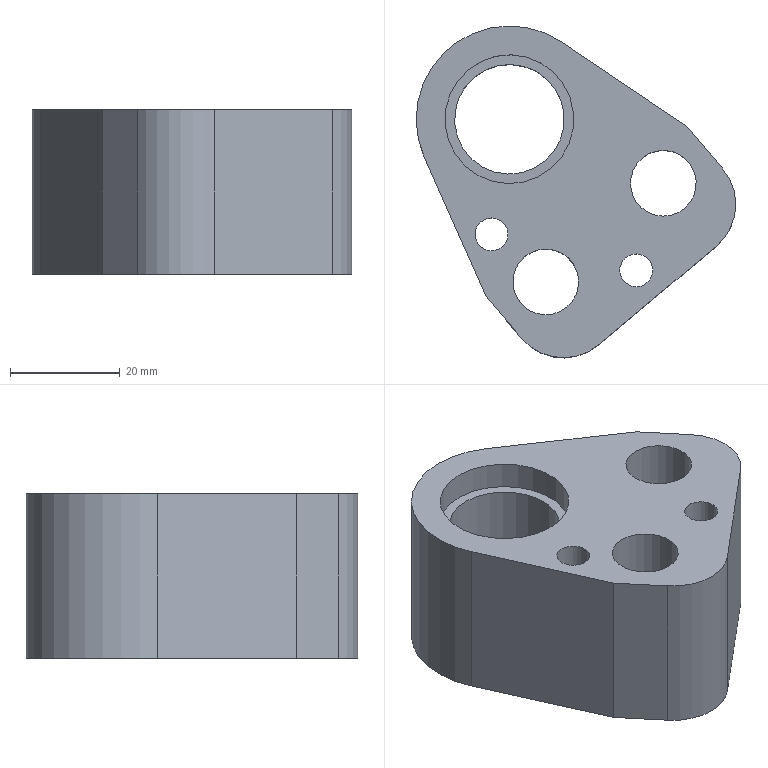Part | NX | features solid 2 | 1 solid | 25 faces | box 58.294 x 60.512 x 30 mm | volume 46591 mm3 | cylinder 13 | plane 12 | commonest cylinder face diameters 20 x3 6 x2 8 x2 12 x2 17 x2 23.5 x1
STEP:
#1=CARTESIAN_POINT('',(142.417,-221.513,161.));
#2=VERTEX_POINT('',#1);
#3=CARTESIAN_POINT('',(144.989,-224.578,161.));
#4=DIRECTION('',(0.,0.,-1.));
#5=DIRECTION('',(-0.6428,0.766,0.));
#6=AXIS2_PLACEMENT_3D('',#3,#4,#5);
#7=CIRCLE('',#6,4.);
#8=EDGE_CURVE('',#2,#2,#7,.F.);
#9=ORIENTED_EDGE('',*,*,#8,.T.);
#10=EDGE_LOOP('',(#9));
#11=FACE_BOUND('',#10,.T.);
#12=CARTESIAN_POINT('',(133.943,-233.194,161.));
#13=VERTEX_POINT('',#12);
#14=CARTESIAN_POINT('',(128.479,-226.682,161.));
#15=DIRECTION('',(0.,0.,1.));
#16=DIRECTION('',(0.6428,-0.766,0.));
#17=AXIS2_PLACEMENT_3D('',#14,#15,#16);
#18=CIRCLE('',#17,8.5);
#19=EDGE_CURVE('',#13,#13,#18,.T.);
#20=ORIENTED_EDGE('',*,*,#19,.T.);
#21=EDGE_LOOP('',(#20));
#22=FACE_BOUND('',#21,.T.);
#23=CARTESIAN_POINT('',(155.392,-215.196,161.));
#24=VERTEX_POINT('',#23);
#25=CARTESIAN_POINT('',(149.928,-208.684,161.));
#26=DIRECTION('',(0.,0.,1.));
#27=DIRECTION('',(0.6428,-0.766,0.));
#28=AXIS2_PLACEMENT_3D('',#25,#26,#27);
#29=CIRCLE('',#28,8.5);
#30=EDGE_CURVE('',#24,#24,#29,.T.);
#31=ORIENTED_EDGE('',*,*,#30,.T.);
#32=EDGE_LOOP('',(#31));
#33=FACE_BOUND('',#32,.T.);
#34=CARTESIAN_POINT('',(115.42,-189.34,161.));
#35=VERTEX_POINT('',#34);
#36=CARTESIAN_POINT('',(121.848,-197.,161.));
#37=DIRECTION('',(0.,0.,-1.));
#38=DIRECTION('',(-0.6428,0.766,0.));
#39=AXIS2_PLACEMENT_3D('',#36,#37,#38);
#40=CIRCLE('',#39,10.);
#41=EDGE_CURVE('',#35,#35,#40,.T.);
#42=ORIENTED_EDGE('',*,*,#41,.F.);
#43=EDGE_LOOP('',(#42));
#44=FACE_BOUND('',#43,.T.);
#45=CARTESIAN_POINT('',(131.351,-182.904,161.));
#46=VERTEX_POINT('',#45);
#47=CARTESIAN_POINT('',(154.375,-198.426,161.));
#48=VERTEX_POINT('',#47);
#49=CARTESIAN_POINT('',(131.351,-182.904,161.));
#50=DIRECTION('',(0.8292,-0.559,0.));
#51=VECTOR('',#50,1000.);
#52=LINE('',#49,#51);
#53=EDGE_CURVE('',#46,#48,#52,.T.);
#54=ORIENTED_EDGE('',*,*,#53,.T.);
#55=CARTESIAN_POINT('',(160.803,-206.087,161.));
#56=VERTEX_POINT('',#55);
#57=CARTESIAN_POINT('',(154.375,-198.426,161.));
#58=DIRECTION('',(0.6428,-0.766,0.));
#59=VECTOR('',#58,1000.);
#60=LINE('',#57,#59);
#61=EDGE_CURVE('',#48,#56,#60,.T.);
#62=ORIENTED_EDGE('',*,*,#61,.T.);
#63=CARTESIAN_POINT('',(159.57,-220.175,161.));
#64=VERTEX_POINT('',#63);
#65=CARTESIAN_POINT('',(153.142,-212.514,161.));
#66=DIRECTION('',(0.,0.,1.));
#67=DIRECTION('',(0.6428,-0.766,0.));
#68=AXIS2_PLACEMENT_3D('',#65,#66,#67);
#69=CIRCLE('',#68,10.);
#70=EDGE_CURVE('',#64,#56,#69,.T.);
#71=ORIENTED_EDGE('',*,*,#70,.F.);
#72=CARTESIAN_POINT('',(138.121,-238.173,161.));
#73=VERTEX_POINT('',#72);
#74=CARTESIAN_POINT('',(159.57,-220.175,161.));
#75=DIRECTION('',(-0.766,-0.6428,0.));
#76=VECTOR('',#75,1000.);
#77=LINE('',#74,#76);
#78=EDGE_CURVE('',#64,#73,#77,.T.);
#79=ORIENTED_EDGE('',*,*,#78,.T.);
#80=CARTESIAN_POINT('',(124.032,-236.94,161.));
#81=VERTEX_POINT('',#80);
#82=CARTESIAN_POINT('',(131.693,-230.512,161.));
#83=DIRECTION('',(0.,0.,1.));
#84=DIRECTION('',(0.6428,-0.766,0.));
#85=AXIS2_PLACEMENT_3D('',#82,#83,#84);
#86=CIRCLE('',#85,10.);
#87=EDGE_CURVE('',#81,#73,#86,.T.);
#88=ORIENTED_EDGE('',*,*,#87,.F.);
#89=CARTESIAN_POINT('',(117.605,-229.28,161.));
#90=VERTEX_POINT('',#89);
#91=CARTESIAN_POINT('',(117.605,-229.28,161.));
#92=DIRECTION('',(0.6428,-0.766,0.));
#93=VECTOR('',#92,1000.);
#94=LINE('',#91,#93);
#95=EDGE_CURVE('',#90,#81,#94,.T.);
#96=ORIENTED_EDGE('',*,*,#95,.F.);
#97=CARTESIAN_POINT('',(106.316,-203.911,161.));
#98=VERTEX_POINT('',#97);
#99=CARTESIAN_POINT('',(106.316,-203.911,161.));
#100=DIRECTION('',(0.4065,-0.9136,0.));
#101=VECTOR('',#100,1000.);
#102=LINE('',#99,#101);
#103=EDGE_CURVE('',#98,#90,#102,.T.);
#104=ORIENTED_EDGE('',*,*,#103,.F.);
#105=CARTESIAN_POINT('',(121.848,-197.,161.));
#106=DIRECTION('',(0.,0.,1.));
#107=DIRECTION('',(0.6428,-0.766,0.));
#108=AXIS2_PLACEMENT_3D('',#105,#106,#107);
#109=CIRCLE('',#108,17.);
#110=EDGE_CURVE('',#46,#98,#109,.T.);
#111=ORIENTED_EDGE('',*,*,#110,.F.);
#112=EDGE_LOOP('',(#54,#62,#71,#79,#88,#96,#104,#111));
#113=FACE_BOUND('',#112,.T.);
#114=CARTESIAN_POINT('',(116.019,-214.945,161.));
#115=VERTEX_POINT('',#114);
#116=CARTESIAN_POINT('',(118.591,-218.009,161.));
#117=DIRECTION('',(0.,0.,-1.));
#118=DIRECTION('',(-0.6428,0.766,0.));
#119=AXIS2_PLACEMENT_3D('',#116,#117,#118);
#120=CIRCLE('',#119,4.);
#121=EDGE_CURVE('',#115,#115,#120,.F.);
#122=ORIENTED_EDGE('',*,*,#121,.T.);
#123=EDGE_LOOP('',(#122));
#124=FACE_BOUND('',#123,.T.);
#125=CARTESIAN_POINT('',(153.142,-212.514,161.));
#126=DIRECTION('',(0.,0.,-1.));
#127=DIRECTION('',(0.6428,-0.766,0.));
#128=AXIS2_PLACEMENT_3D('',#125,#126,#127);
#129=PLANE('',#128);
#130=ADVANCED_FACE('',(#11,#22,#33,#44,#113,#124),#129,.T.);
#131=CARTESIAN_POINT('',(146.917,-226.876,191.));
#132=VERTEX_POINT('',#131);
#133=CARTESIAN_POINT('',(144.989,-224.578,191.));
#134=DIRECTION('',(0.,0.,1.));
#135=DIRECTION('',(0.6428,-0.766,0.));
#136=AXIS2_PLACEMENT_3D('',#133,#134,#135);
#137=CIRCLE('',#136,3.);
#138=EDGE_CURVE('',#132,#132,#137,.T.);
#139=ORIENTED_EDGE('',*,*,#138,.T.);
#140=EDGE_LOOP('',(#139));
#141=FACE_BOUND('',#140,.T.);
#142=CARTESIAN_POINT('',(146.917,-226.876,181.));
#143=VERTEX_POINT('',#142);
#144=CARTESIAN_POINT('',(144.989,-224.578,181.));
#145=DIRECTION('',(0.,0.,1.));
#146=DIRECTION('',(0.6428,-0.766,0.));
#147=AXIS2_PLACEMENT_3D('',#144,#145,#146);
#148=CIRCLE('',#147,3.);
#149=EDGE_CURVE('',#143,#143,#148,.T.);
#150=ORIENTED_EDGE('',*,*,#149,.F.);
#151=EDGE_LOOP('',(#150));
#152=FACE_BOUND('',#151,.T.);
#153=CARTESIAN_POINT('',(144.989,-224.578,161.));
#154=DIRECTION('',(0.,0.,1.));
#155=DIRECTION('',(-0.6428,0.766,0.));
#156=AXIS2_PLACEMENT_3D('',#153,#154,#155);
#157=CYLINDRICAL_SURFACE('',#156,3.);
#158=ADVANCED_FACE('',(#141,#152),#157,.F.);
#159=CARTESIAN_POINT('',(132.336,-231.278,191.));
#160=VERTEX_POINT('',#159);
#161=CARTESIAN_POINT('',(128.479,-226.682,191.));
#162=DIRECTION('',(0.,0.,1.));
#163=DIRECTION('',(0.6428,-0.766,0.));
#164=AXIS2_PLACEMENT_3D('',#161,#162,#163);
#165=CIRCLE('',#164,6.);
#166=EDGE_CURVE('',#160,#160,#165,.T.);
#167=ORIENTED_EDGE('',*,*,#166,.T.);
#168=EDGE_LOOP('',(#167));
#169=FACE_BOUND('',#168,.T.);
#170=CARTESIAN_POINT('',(132.336,-231.278,173.));
#171=VERTEX_POINT('',#170);
#172=CARTESIAN_POINT('',(128.479,-226.682,173.));
#173=DIRECTION('',(0.,0.,1.));
#174=DIRECTION('',(0.6428,-0.766,0.));
#175=AXIS2_PLACEMENT_3D('',#172,#173,#174);
#176=CIRCLE('',#175,6.);
#177=EDGE_CURVE('',#171,#171,#176,.T.);
#178=ORIENTED_EDGE('',*,*,#177,.F.);
#179=EDGE_LOOP('',(#178));
#180=FACE_BOUND('',#179,.T.);
#181=CARTESIAN_POINT('',(128.479,-226.682,161.));
#182=DIRECTION('',(0.,0.,1.));
#183=DIRECTION('',(-0.6428,0.766,0.));
#184=AXIS2_PLACEMENT_3D('',#181,#182,#183);
#185=CYLINDRICAL_SURFACE('',#184,6.);
#186=ADVANCED_FACE('',(#169,#180),#185,.F.);
#187=CARTESIAN_POINT('',(153.785,-213.28,191.));
#188=VERTEX_POINT('',#187);
#189=CARTESIAN_POINT('',(149.928,-208.684,191.));
#190=DIRECTION('',(0.,0.,1.));
#191=DIRECTION('',(0.6428,-0.766,0.));
#192=AXIS2_PLACEMENT_3D('',#189,#190,#191);
#193=CIRCLE('',#192,6.);
#194=EDGE_CURVE('',#188,#188,#193,.T.);
#195=ORIENTED_EDGE('',*,*,#194,.T.);
#196=EDGE_LOOP('',(#195));
#197=FACE_BOUND('',#196,.T.);
#198=CARTESIAN_POINT('',(153.785,-213.28,173.));
#199=VERTEX_POINT('',#198);
#200=CARTESIAN_POINT('',(149.928,-208.684,173.));
#201=DIRECTION('',(0.,0.,1.));
#202=DIRECTION('',(0.6428,-0.766,0.));
#203=AXIS2_PLACEMENT_3D('',#200,#201,#202);
#204=CIRCLE('',#203,6.);
#205=EDGE_CURVE('',#199,#199,#204,.T.);
#206=ORIENTED_EDGE('',*,*,#205,.F.);
#207=EDGE_LOOP('',(#206));
#208=FACE_BOUND('',#207,.T.);
#209=CARTESIAN_POINT('',(149.928,-208.684,161.));
#210=DIRECTION('',(0.,0.,1.));
#211=DIRECTION('',(-0.6428,0.766,0.));
#212=AXIS2_PLACEMENT_3D('',#209,#210,#211);
#213=CYLINDRICAL_SURFACE('',#212,6.);
#214=ADVANCED_FACE('',(#197,#208),#213,.F.);
#215=CARTESIAN_POINT('',(120.519,-220.307,191.));
#216=VERTEX_POINT('',#215);
#217=CARTESIAN_POINT('',(118.591,-218.009,191.));
#218=DIRECTION('',(0.,0.,1.));
#219=DIRECTION('',(0.6428,-0.766,0.));
#220=AXIS2_PLACEMENT_3D('',#217,#218,#219);
#221=CIRCLE('',#220,3.);
#222=EDGE_CURVE('',#216,#216,#221,.T.);
#223=ORIENTED_EDGE('',*,*,#222,.F.);
#224=EDGE_LOOP('',(#223));
#225=FACE_BOUND('',#224,.T.);
#226=ORIENTED_EDGE('',*,*,#166,.F.);
#227=EDGE_LOOP('',(#226));
#228=FACE_BOUND('',#227,.T.);
#229=CARTESIAN_POINT('',(131.351,-182.904,191.));
#230=VERTEX_POINT('',#229);
#231=CARTESIAN_POINT('',(154.375,-198.426,191.));
#232=VERTEX_POINT('',#231);
#233=CARTESIAN_POINT('',(131.351,-182.904,191.));
#234=DIRECTION('',(0.8292,-0.559,0.));
#235=VECTOR('',#234,1000.);
#236=LINE('',#233,#235);
#237=EDGE_CURVE('',#230,#232,#236,.T.);
#238=ORIENTED_EDGE('',*,*,#237,.F.);
#239=CARTESIAN_POINT('',(106.316,-203.911,191.));
#240=VERTEX_POINT('',#239);
#241=CARTESIAN_POINT('',(121.848,-197.,191.));
#242=DIRECTION('',(0.,0.,1.));
#243=DIRECTION('',(0.6428,-0.766,0.));
#244=AXIS2_PLACEMENT_3D('',#241,#242,#243);
#245=CIRCLE('',#244,17.);
#246=EDGE_CURVE('',#230,#240,#245,.T.);
#247=ORIENTED_EDGE('',*,*,#246,.T.);
#248=CARTESIAN_POINT('',(117.605,-229.28,191.));
#249=VERTEX_POINT('',#248);
#250=CARTESIAN_POINT('',(106.316,-203.911,191.));
#251=DIRECTION('',(0.4065,-0.9136,0.));
#252=VECTOR('',#251,1000.);
#253=LINE('',#250,#252);
#254=EDGE_CURVE('',#240,#249,#253,.T.);
#255=ORIENTED_EDGE('',*,*,#254,.T.);
#256=CARTESIAN_POINT('',(124.032,-236.94,191.));
#257=VERTEX_POINT('',#256);
#258=CARTESIAN_POINT('',(117.605,-229.28,191.));
#259=DIRECTION('',(0.6428,-0.766,0.));
#260=VECTOR('',#259,1000.);
#261=LINE('',#258,#260);
#262=EDGE_CURVE('',#249,#257,#261,.T.);
#263=ORIENTED_EDGE('',*,*,#262,.T.);
#264=CARTESIAN_POINT('',(138.121,-238.173,191.));
#265=VERTEX_POINT('',#264);
#266=CARTESIAN_POINT('',(131.693,-230.512,191.));
#267=DIRECTION('',(0.,0.,1.));
#268=DIRECTION('',(0.6428,-0.766,0.));
#269=AXIS2_PLACEMENT_3D('',#266,#267,#268);
#270=CIRCLE('',#269,10.);
#271=EDGE_CURVE('',#257,#265,#270,.T.);
#272=ORIENTED_EDGE('',*,*,#271,.T.);
#273=CARTESIAN_POINT('',(159.57,-220.175,191.));
#274=VERTEX_POINT('',#273);
#275=CARTESIAN_POINT('',(159.57,-220.175,191.));
#276=DIRECTION('',(-0.766,-0.6428,0.));
#277=VECTOR('',#276,1000.);
#278=LINE('',#275,#277);
#279=EDGE_CURVE('',#274,#265,#278,.T.);
#280=ORIENTED_EDGE('',*,*,#279,.F.);
#281=CARTESIAN_POINT('',(160.803,-206.087,191.));
#282=VERTEX_POINT('',#281);
#283=CARTESIAN_POINT('',(153.142,-212.514,191.));
#284=DIRECTION('',(0.,0.,1.));
#285=DIRECTION('',(0.6428,-0.766,0.));
#286=AXIS2_PLACEMENT_3D('',#283,#284,#285);
#287=CIRCLE('',#286,10.);
#288=EDGE_CURVE('',#274,#282,#287,.T.);
#289=ORIENTED_EDGE('',*,*,#288,.T.);
#290=CARTESIAN_POINT('',(154.375,-198.426,191.));
#291=DIRECTION('',(0.6428,-0.766,0.));
#292=VECTOR('',#291,1000.);
#293=LINE('',#290,#292);
#294=EDGE_CURVE('',#232,#282,#293,.T.);
#295=ORIENTED_EDGE('',*,*,#294,.F.);
#296=EDGE_LOOP('',(#238,#247,#255,#263,#272,#280,#289,#295));
#297=FACE_BOUND('',#296,.T.);
#298=CARTESIAN_POINT('',(129.401,-206.001,191.));
#299=VERTEX_POINT('',#298);
#300=CARTESIAN_POINT('',(121.848,-197.,191.));
#301=DIRECTION('',(0.,0.,1.));
#302=DIRECTION('',(0.6428,-0.766,0.));
#303=AXIS2_PLACEMENT_3D('',#300,#301,#302);
#304=CIRCLE('',#303,11.75);
#305=EDGE_CURVE('',#299,#299,#304,.T.);
#306=ORIENTED_EDGE('',*,*,#305,.F.);
#307=EDGE_LOOP('',(#306));
#308=FACE_BOUND('',#307,.T.);
#309=ORIENTED_EDGE('',*,*,#194,.F.);
#310=EDGE_LOOP('',(#309));
#311=FACE_BOUND('',#310,.T.);
#312=ORIENTED_EDGE('',*,*,#138,.F.);
#313=EDGE_LOOP('',(#312));
#314=FACE_BOUND('',#313,.T.);
#315=CARTESIAN_POINT('',(153.142,-212.514,191.));
#316=DIRECTION('',(0.,0.,-1.));
#317=DIRECTION('',(0.6428,-0.766,0.));
#318=AXIS2_PLACEMENT_3D('',#315,#316,#317);
#319=PLANE('',#318);
#320=ADVANCED_FACE('',(#225,#228,#297,#308,#311,#314),#319,.F.);
#321=ORIENTED_EDGE('',*,*,#237,.T.);
#322=CARTESIAN_POINT('',(154.375,-198.426,161.));
#323=DIRECTION('',(0.,0.,1.));
#324=VECTOR('',#323,1000.);
#325=LINE('',#322,#324);
#326=EDGE_CURVE('',#48,#232,#325,.T.);
#327=ORIENTED_EDGE('',*,*,#326,.F.);
#328=ORIENTED_EDGE('',*,*,#53,.F.);
#329=CARTESIAN_POINT('',(131.351,-182.904,161.));
#330=DIRECTION('',(0.,0.,1.));
#331=VECTOR('',#330,1000.);
#332=LINE('',#329,#331);
#333=EDGE_CURVE('',#46,#230,#332,.T.);
#334=ORIENTED_EDGE('',*,*,#333,.T.);
#335=EDGE_LOOP('',(#321,#327,#328,#334));
#336=FACE_BOUND('',#335,.T.);
#337=CARTESIAN_POINT('',(131.351,-182.904,161.));
#338=DIRECTION('',(0.559,0.8292,0.));
#339=DIRECTION('',(0.8292,-0.559,0.));
#340=AXIS2_PLACEMENT_3D('',#337,#338,#339);
#341=PLANE('',#340);
#342=ADVANCED_FACE('',(#336),#341,.T.);
#343=ORIENTED_EDGE('',*,*,#294,.T.);
#344=CARTESIAN_POINT('',(160.803,-206.087,161.));
#345=DIRECTION('',(0.,0.,1.));
#346=VECTOR('',#345,1000.);
#347=LINE('',#344,#346);
#348=EDGE_CURVE('',#56,#282,#347,.T.);
#349=ORIENTED_EDGE('',*,*,#348,.F.);
#350=ORIENTED_EDGE('',*,*,#61,.F.);
#351=ORIENTED_EDGE('',*,*,#326,.T.);
#352=EDGE_LOOP('',(#343,#349,#350,#351));
#353=FACE_BOUND('',#352,.T.);
#354=CARTESIAN_POINT('',(154.375,-198.426,161.));
#355=DIRECTION('',(0.766,0.6428,0.));
#356=DIRECTION('',(0.6428,-0.766,0.));
#357=AXIS2_PLACEMENT_3D('',#354,#355,#356);
#358=PLANE('',#357);
#359=ADVANCED_FACE('',(#353),#358,.T.);
#360=ORIENTED_EDGE('',*,*,#288,.F.);
#361=CARTESIAN_POINT('',(159.57,-220.175,161.));
#362=DIRECTION('',(0.,0.,1.));
#363=VECTOR('',#362,1000.);
#364=LINE('',#361,#363);
#365=EDGE_CURVE('',#64,#274,#364,.T.);
#366=ORIENTED_EDGE('',*,*,#365,.F.);
#367=ORIENTED_EDGE('',*,*,#70,.T.);
#368=ORIENTED_EDGE('',*,*,#348,.T.);
#369=EDGE_LOOP('',(#360,#366,#367,#368));
#370=FACE_BOUND('',#369,.T.);
#371=CARTESIAN_POINT('',(153.142,-212.514,161.));
#372=DIRECTION('',(0.,0.,1.));
#373=DIRECTION('',(-0.6428,0.766,0.));
#374=AXIS2_PLACEMENT_3D('',#371,#372,#373);
#375=CYLINDRICAL_SURFACE('',#374,10.);
#376=ADVANCED_FACE('',(#370),#375,.T.);
#377=ORIENTED_EDGE('',*,*,#279,.T.);
#378=CARTESIAN_POINT('',(138.121,-238.173,161.));
#379=DIRECTION('',(0.,0.,1.));
#380=VECTOR('',#379,1000.);
#381=LINE('',#378,#380);
#382=EDGE_CURVE('',#73,#265,#381,.T.);
#383=ORIENTED_EDGE('',*,*,#382,.F.);
#384=ORIENTED_EDGE('',*,*,#78,.F.);
#385=ORIENTED_EDGE('',*,*,#365,.T.);
#386=EDGE_LOOP('',(#377,#383,#384,#385));
#387=FACE_BOUND('',#386,.T.);
#388=CARTESIAN_POINT('',(159.57,-220.175,161.));
#389=DIRECTION('',(0.6428,-0.766,0.));
#390=DIRECTION('',(-0.766,-0.6428,0.));
#391=AXIS2_PLACEMENT_3D('',#388,#389,#390);
#392=PLANE('',#391);
#393=ADVANCED_FACE('',(#387),#392,.T.);
#394=ORIENTED_EDGE('',*,*,#271,.F.);
#395=CARTESIAN_POINT('',(124.032,-236.94,161.));
#396=DIRECTION('',(0.,0.,1.));
#397=VECTOR('',#396,1000.);
#398=LINE('',#395,#397);
#399=EDGE_CURVE('',#81,#257,#398,.T.);
#400=ORIENTED_EDGE('',*,*,#399,.F.);
#401=ORIENTED_EDGE('',*,*,#87,.T.);
#402=ORIENTED_EDGE('',*,*,#382,.T.);
#403=EDGE_LOOP('',(#394,#400,#401,#402));
#404=FACE_BOUND('',#403,.T.);
#405=CARTESIAN_POINT('',(131.693,-230.512,161.));
#406=DIRECTION('',(0.,0.,1.));
#407=DIRECTION('',(-0.6428,0.766,0.));
#408=AXIS2_PLACEMENT_3D('',#405,#406,#407);
#409=CYLINDRICAL_SURFACE('',#408,10.);
#410=ADVANCED_FACE('',(#404),#409,.T.);
#411=ORIENTED_EDGE('',*,*,#262,.F.);
#412=CARTESIAN_POINT('',(117.605,-229.28,161.));
#413=DIRECTION('',(0.,0.,1.));
#414=VECTOR('',#413,1000.);
#415=LINE('',#412,#414);
#416=EDGE_CURVE('',#90,#249,#415,.T.);
#417=ORIENTED_EDGE('',*,*,#416,.F.);
#418=ORIENTED_EDGE('',*,*,#95,.T.);
#419=ORIENTED_EDGE('',*,*,#399,.T.);
#420=EDGE_LOOP('',(#411,#417,#418,#419));
#421=FACE_BOUND('',#420,.T.);
#422=CARTESIAN_POINT('',(117.605,-229.28,161.));
#423=DIRECTION('',(0.766,0.6428,0.));
#424=DIRECTION('',(0.,0.,1.));
#425=AXIS2_PLACEMENT_3D('',#422,#423,#424);
#426=PLANE('',#425);
#427=ADVANCED_FACE('',(#421),#426,.F.);
#428=ORIENTED_EDGE('',*,*,#254,.F.);
#429=CARTESIAN_POINT('',(106.316,-203.911,161.));
#430=DIRECTION('',(0.,0.,1.));
#431=VECTOR('',#430,1000.);
#432=LINE('',#429,#431);
#433=EDGE_CURVE('',#98,#240,#432,.T.);
#434=ORIENTED_EDGE('',*,*,#433,.F.);
#435=ORIENTED_EDGE('',*,*,#103,.T.);
#436=ORIENTED_EDGE('',*,*,#416,.T.);
#437=EDGE_LOOP('',(#428,#434,#435,#436));
#438=FACE_BOUND('',#437,.T.);
#439=CARTESIAN_POINT('',(106.316,-203.911,161.));
#440=DIRECTION('',(0.9136,0.4065,0.));
#441=DIRECTION('',(0.4065,-0.9136,0.));
#442=AXIS2_PLACEMENT_3D('',#439,#440,#441);
#443=PLANE('',#442);
#444=ADVANCED_FACE('',(#438),#443,.F.);
#445=ORIENTED_EDGE('',*,*,#246,.F.);
#446=ORIENTED_EDGE('',*,*,#333,.F.);
#447=ORIENTED_EDGE('',*,*,#110,.T.);
#448=ORIENTED_EDGE('',*,*,#433,.T.);
#449=EDGE_LOOP('',(#445,#446,#447,#448));
#450=FACE_BOUND('',#449,.T.);
#451=CARTESIAN_POINT('',(121.848,-197.,161.));
#452=DIRECTION('',(0.,0.,1.));
#453=DIRECTION('',(-0.6428,0.766,0.));
#454=AXIS2_PLACEMENT_3D('',#451,#452,#453);
#455=CYLINDRICAL_SURFACE('',#454,17.);
#456=ADVANCED_FACE('',(#450),#455,.T.);
#457=CARTESIAN_POINT('',(128.276,-204.66,186.));
#458=VERTEX_POINT('',#457);
#459=CARTESIAN_POINT('',(121.848,-197.,186.));
#460=DIRECTION('',(0.,0.,1.));
#461=DIRECTION('',(0.6428,-0.766,0.));
#462=AXIS2_PLACEMENT_3D('',#459,#460,#461);
#463=CIRCLE('',#462,10.);
#464=EDGE_CURVE('',#458,#458,#463,.F.);
#465=ORIENTED_EDGE('',*,*,#464,.F.);
#466=EDGE_LOOP('',(#465));
#467=FACE_BOUND('',#466,.T.);
#468=ORIENTED_EDGE('',*,*,#41,.T.);
#469=EDGE_LOOP('',(#468));
#470=FACE_BOUND('',#469,.T.);
#471=CARTESIAN_POINT('',(121.848,-197.,161.));
#472=DIRECTION('',(0.,0.,1.));
#473=DIRECTION('',(-0.6428,0.766,0.));
#474=AXIS2_PLACEMENT_3D('',#471,#472,#473);
#475=CYLINDRICAL_SURFACE('',#474,10.);
#476=ADVANCED_FACE('',(#467,#470),#475,.F.);
#477=CARTESIAN_POINT('',(129.401,-206.001,186.));
#478=VERTEX_POINT('',#477);
#479=CARTESIAN_POINT('',(121.848,-197.,186.));
#480=DIRECTION('',(0.,0.,1.));
#481=DIRECTION('',(0.6428,-0.766,0.));
#482=AXIS2_PLACEMENT_3D('',#479,#480,#481);
#483=CIRCLE('',#482,11.75);
#484=EDGE_CURVE('',#478,#478,#483,.T.);
#485=ORIENTED_EDGE('',*,*,#484,.T.);
#486=EDGE_LOOP('',(#485));
#487=FACE_BOUND('',#486,.T.);
#488=ORIENTED_EDGE('',*,*,#464,.T.);
#489=EDGE_LOOP('',(#488));
#490=FACE_BOUND('',#489,.T.);
#491=CARTESIAN_POINT('',(121.848,-197.,186.));
#492=DIRECTION('',(0.,0.,-1.));
#493=DIRECTION('',(0.6428,-0.766,0.));
#494=AXIS2_PLACEMENT_3D('',#491,#492,#493);
#495=PLANE('',#494);
#496=ADVANCED_FACE('',(#487,#490),#495,.F.);
#497=ORIENTED_EDGE('',*,*,#484,.F.);
#498=EDGE_LOOP('',(#497));
#499=FACE_BOUND('',#498,.T.);
#500=ORIENTED_EDGE('',*,*,#305,.T.);
#501=EDGE_LOOP('',(#500));
#502=FACE_BOUND('',#501,.T.);
#503=CARTESIAN_POINT('',(121.848,-197.,186.));
#504=DIRECTION('',(0.,0.,1.));
#505=DIRECTION('',(-0.6428,0.766,0.));
#506=AXIS2_PLACEMENT_3D('',#503,#504,#505);
#507=CYLINDRICAL_SURFACE('',#506,11.75);
#508=ADVANCED_FACE('',(#499,#502),#507,.F.);
#509=CARTESIAN_POINT('',(120.519,-220.307,181.));
#510=VERTEX_POINT('',#509);
#511=CARTESIAN_POINT('',(118.591,-218.009,181.));
#512=DIRECTION('',(0.,0.,1.));
#513=DIRECTION('',(0.6428,-0.766,0.));
#514=AXIS2_PLACEMENT_3D('',#511,#512,#513);
#515=CIRCLE('',#514,3.);
#516=EDGE_CURVE('',#510,#510,#515,.T.);
#517=ORIENTED_EDGE('',*,*,#516,.F.);
#518=EDGE_LOOP('',(#517));
#519=FACE_BOUND('',#518,.T.);
#520=ORIENTED_EDGE('',*,*,#222,.T.);
#521=EDGE_LOOP('',(#520));
#522=FACE_BOUND('',#521,.T.);
#523=CARTESIAN_POINT('',(118.591,-218.009,161.));
#524=DIRECTION('',(0.,0.,1.));
#525=DIRECTION('',(-0.6428,0.766,0.));
#526=AXIS2_PLACEMENT_3D('',#523,#524,#525);
#527=CYLINDRICAL_SURFACE('',#526,3.);
#528=ADVANCED_FACE('',(#519,#522),#527,.F.);
#529=CARTESIAN_POINT('',(155.392,-215.196,173.));
#530=VERTEX_POINT('',#529);
#531=CARTESIAN_POINT('',(149.928,-208.684,173.));
#532=DIRECTION('',(0.,0.,1.));
#533=DIRECTION('',(0.6428,-0.766,0.));
#534=AXIS2_PLACEMENT_3D('',#531,#532,#533);
#535=CIRCLE('',#534,8.5);
#536=EDGE_CURVE('',#530,#530,#535,.T.);
#537=ORIENTED_EDGE('',*,*,#536,.T.);
#538=EDGE_LOOP('',(#537));
#539=FACE_BOUND('',#538,.T.);
#540=ORIENTED_EDGE('',*,*,#30,.F.);
#541=EDGE_LOOP('',(#540));
#542=FACE_BOUND('',#541,.T.);
#543=CARTESIAN_POINT('',(149.928,-208.684,173.));
#544=DIRECTION('',(0.,0.,-1.));
#545=DIRECTION('',(0.6428,-0.766,0.));
#546=AXIS2_PLACEMENT_3D('',#543,#544,#545);
#547=CYLINDRICAL_SURFACE('',#546,8.5);
#548=ADVANCED_FACE('',(#539,#542),#547,.F.);
#549=ORIENTED_EDGE('',*,*,#205,.T.);
#550=EDGE_LOOP('',(#549));
#551=FACE_BOUND('',#550,.T.);
#552=ORIENTED_EDGE('',*,*,#536,.F.);
#553=EDGE_LOOP('',(#552));
#554=FACE_BOUND('',#553,.T.);
#555=CARTESIAN_POINT('',(149.928,-208.684,173.));
#556=DIRECTION('',(0.,0.,-1.));
#557=DIRECTION('',(0.6428,-0.766,0.));
#558=AXIS2_PLACEMENT_3D('',#555,#556,#557);
#559=PLANE('',#558);
#560=ADVANCED_FACE('',(#551,#554),#559,.T.);
#561=CARTESIAN_POINT('',(133.943,-233.194,173.));
#562=VERTEX_POINT('',#561);
#563=CARTESIAN_POINT('',(128.479,-226.682,173.));
#564=DIRECTION('',(0.,0.,1.));
#565=DIRECTION('',(0.6428,-0.766,0.));
#566=AXIS2_PLACEMENT_3D('',#563,#564,#565);
#567=CIRCLE('',#566,8.5);
#568=EDGE_CURVE('',#562,#562,#567,.T.);
#569=ORIENTED_EDGE('',*,*,#568,.T.);
#570=EDGE_LOOP('',(#569));
#571=FACE_BOUND('',#570,.T.);
#572=ORIENTED_EDGE('',*,*,#19,.F.);
#573=EDGE_LOOP('',(#572));
#574=FACE_BOUND('',#573,.T.);
#575=CARTESIAN_POINT('',(128.479,-226.682,173.));
#576=DIRECTION('',(0.,0.,-1.));
#577=DIRECTION('',(0.6428,-0.766,0.));
#578=AXIS2_PLACEMENT_3D('',#575,#576,#577);
#579=CYLINDRICAL_SURFACE('',#578,8.5);
#580=ADVANCED_FACE('',(#571,#574),#579,.F.);
#581=ORIENTED_EDGE('',*,*,#177,.T.);
#582=EDGE_LOOP('',(#581));
#583=FACE_BOUND('',#582,.T.);
#584=ORIENTED_EDGE('',*,*,#568,.F.);
#585=EDGE_LOOP('',(#584));
#586=FACE_BOUND('',#585,.T.);
#587=CARTESIAN_POINT('',(128.479,-226.682,173.));
#588=DIRECTION('',(0.,0.,-1.));
#589=DIRECTION('',(0.6428,-0.766,0.));
#590=AXIS2_PLACEMENT_3D('',#587,#588,#589);
#591=PLANE('',#590);
#592=ADVANCED_FACE('',(#583,#586),#591,.T.);
#593=ORIENTED_EDGE('',*,*,#149,.T.);
#594=EDGE_LOOP('',(#593));
#595=FACE_BOUND('',#594,.T.);
#596=CARTESIAN_POINT('',(142.417,-221.513,181.));
#597=VERTEX_POINT('',#596);
#598=CARTESIAN_POINT('',(144.989,-224.578,181.));
#599=DIRECTION('',(0.,0.,-1.));
#600=DIRECTION('',(-0.6428,0.766,0.));
#601=AXIS2_PLACEMENT_3D('',#598,#599,#600);
#602=CIRCLE('',#601,4.);
#603=EDGE_CURVE('',#597,#597,#602,.F.);
#604=ORIENTED_EDGE('',*,*,#603,.F.);
#605=EDGE_LOOP('',(#604));
#606=FACE_BOUND('',#605,.T.);
#607=CARTESIAN_POINT('',(144.989,-224.578,181.));
#608=DIRECTION('',(0.,0.,1.));
#609=DIRECTION('',(-0.6428,0.766,0.));
#610=AXIS2_PLACEMENT_3D('',#607,#608,#609);
#611=PLANE('',#610);
#612=ADVANCED_FACE('',(#595,#606),#611,.F.);
#613=ORIENTED_EDGE('',*,*,#603,.T.);
#614=EDGE_LOOP('',(#613));
#615=FACE_BOUND('',#614,.T.);
#616=ORIENTED_EDGE('',*,*,#8,.F.);
#617=EDGE_LOOP('',(#616));
#618=FACE_BOUND('',#617,.T.);
#619=CARTESIAN_POINT('',(144.989,-224.578,161.));
#620=DIRECTION('',(0.,0.,1.));
#621=DIRECTION('',(-0.6428,0.766,0.));
#622=AXIS2_PLACEMENT_3D('',#619,#620,#621);
#623=CYLINDRICAL_SURFACE('',#622,4.);
#624=ADVANCED_FACE('',(#615,#618),#623,.F.);
#625=ORIENTED_EDGE('',*,*,#516,.T.);
#626=EDGE_LOOP('',(#625));
#627=FACE_BOUND('',#626,.T.);
#628=CARTESIAN_POINT('',(116.019,-214.945,181.));
#629=VERTEX_POINT('',#628);
#630=CARTESIAN_POINT('',(118.591,-218.009,181.));
#631=DIRECTION('',(0.,0.,-1.));
#632=DIRECTION('',(-0.6428,0.766,0.));
#633=AXIS2_PLACEMENT_3D('',#630,#631,#632);
#634=CIRCLE('',#633,4.);
#635=EDGE_CURVE('',#629,#629,#634,.F.);
#636=ORIENTED_EDGE('',*,*,#635,.F.);
#637=EDGE_LOOP('',(#636));
#638=FACE_BOUND('',#637,.T.);
#639=CARTESIAN_POINT('',(118.591,-218.009,181.));
#640=DIRECTION('',(0.,0.,1.));
#641=DIRECTION('',(-0.6428,0.766,0.));
#642=AXIS2_PLACEMENT_3D('',#639,#640,#641);
#643=PLANE('',#642);
#644=ADVANCED_FACE('',(#627,#638),#643,.F.);
#645=ORIENTED_EDGE('',*,*,#635,.T.);
#646=EDGE_LOOP('',(#645));
#647=FACE_BOUND('',#646,.T.);
#648=ORIENTED_EDGE('',*,*,#121,.F.);
#649=EDGE_LOOP('',(#648));
#650=FACE_BOUND('',#649,.T.);
#651=CARTESIAN_POINT('',(118.591,-218.009,161.));
#652=DIRECTION('',(0.,0.,1.));
#653=DIRECTION('',(-0.6428,0.766,0.));
#654=AXIS2_PLACEMENT_3D('',#651,#652,#653);
#655=CYLINDRICAL_SURFACE('',#654,4.);
#656=ADVANCED_FACE('',(#647,#650),#655,.F.);
#657=CLOSED_SHELL('',(#130,#158,#186,#214,#320,#342,#359,#376,#393,#410,#427,#444,#456,#476,#496,#508,#528,#548,#560,#580,#592,#612,#624,#644,#656));
#658=MANIFOLD_SOLID_BREP('',#657);
#659=(LENGTH_UNIT()NAMED_UNIT(*)SI_UNIT(.MILLI.,.METRE.));
#660=UNCERTAINTY_MEASURE_WITH_UNIT(LENGTH_MEASURE(0.00001),#659,'','');
#661=(NAMED_UNIT(*)PLANE_ANGLE_UNIT()SI_UNIT($,.RADIAN.));
#662=(NAMED_UNIT(*)SI_UNIT($,.STERADIAN.)SOLID_ANGLE_UNIT());
#663=(GEOMETRIC_REPRESENTATION_CONTEXT(3)GLOBAL_UNCERTAINTY_ASSIGNED_CONTEXT((#660))GLOBAL_UNIT_ASSIGNED_CONTEXT((#659,#661,#662))REPRESENTATION_CONTEXT('',''));
#664=ADVANCED_BREP_SHAPE_REPRESENTATION('',(#658),#663);